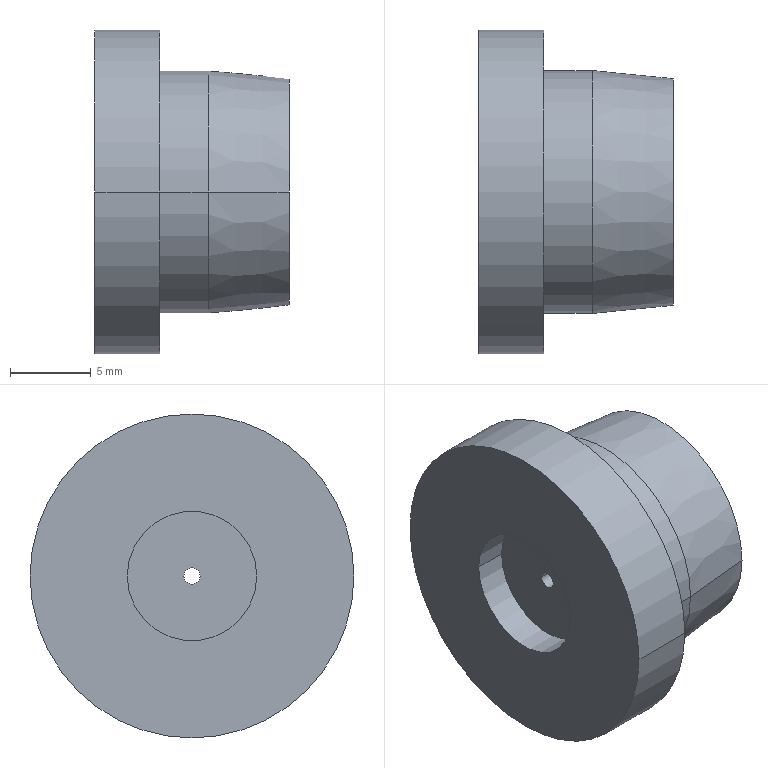Part | SolidWorks | features ICE 3, RevCut 1, Revolution 1 | 1 solid | 19 faces | box 12 x 20 x 20 mm | volume 1878 mm3 | cylinder 10 | plane 5 | sphere 2 | cone 2 | commonest cylinder face diameters 1 x2 4 x2 8 x2 15 x2 20 x2
STEP:
#1=CARTESIAN_POINT('',(12.,-5.809,0.));
#2=VERTEX_POINT('',#1);
#3=CARTESIAN_POINT('',(12.,5.809,0.));
#4=VERTEX_POINT('',#3);
#5=CARTESIAN_POINT('',(12.,0.,0.));
#6=DIRECTION('',(-1.,0.,0.));
#7=DIRECTION('',(0.,1.,0.));
#8=AXIS2_PLACEMENT_3D('',#5,#6,#7);
#9=CIRCLE('',#8,5.809);
#10=EDGE_CURVE('',#2,#4,#9,.T.);
#11=ORIENTED_EDGE('',*,*,#10,.F.);
#12=CARTESIAN_POINT('',(4.843,-2.,0.));
#13=VERTEX_POINT('',#12);
#14=CARTESIAN_POINT('',(10.5,0.,0.));
#15=DIRECTION('',(0.,0.,-1.));
#16=DIRECTION('',(0.,1.,0.));
#17=AXIS2_PLACEMENT_3D('',#14,#15,#16);
#18=CIRCLE('',#17,6.);
#19=EDGE_CURVE('',#2,#13,#18,.T.);
#20=ORIENTED_EDGE('',*,*,#19,.T.);
#21=CARTESIAN_POINT('',(4.843,2.,0.));
#22=VERTEX_POINT('',#21);
#23=CARTESIAN_POINT('',(4.843,0.,0.));
#24=DIRECTION('',(-1.,0.,0.));
#25=DIRECTION('',(0.,1.,0.));
#26=AXIS2_PLACEMENT_3D('',#23,#24,#25);
#27=CIRCLE('',#26,2.);
#28=EDGE_CURVE('',#13,#22,#27,.T.);
#29=ORIENTED_EDGE('',*,*,#28,.T.);
#30=CARTESIAN_POINT('',(10.5,0.,0.));
#31=DIRECTION('',(0.,0.,1.));
#32=DIRECTION('',(0.,-1.,0.));
#33=AXIS2_PLACEMENT_3D('',#30,#31,#32);
#34=CIRCLE('',#33,6.);
#35=EDGE_CURVE('',#4,#22,#34,.T.);
#36=ORIENTED_EDGE('',*,*,#35,.F.);
#37=EDGE_LOOP('',(#11,#20,#29,#36));
#38=FACE_OUTER_BOUND('',#37,.T.);
#39=CARTESIAN_POINT('',(10.5,0.,0.));
#40=DIRECTION('',(0.,0.,-1.));
#41=DIRECTION('',(0.,1.,0.));
#42=AXIS2_PLACEMENT_3D('',#39,#40,#41);
#43=SPHERICAL_SURFACE('',#42,6.);
#44=ADVANCED_FACE('',(#38),#43,.F.);
#45=CARTESIAN_POINT('',(3.5,-0.5,0.));
#46=VERTEX_POINT('',#45);
#47=CARTESIAN_POINT('',(3.5,0.5,0.));
#48=VERTEX_POINT('',#47);
#49=CARTESIAN_POINT('',(3.5,0.,0.));
#50=DIRECTION('',(1.,0.,0.));
#51=DIRECTION('',(0.,-1.,0.));
#52=AXIS2_PLACEMENT_3D('',#49,#50,#51);
#53=CIRCLE('',#52,0.5);
#54=EDGE_CURVE('',#46,#48,#53,.T.);
#55=ORIENTED_EDGE('',*,*,#54,.T.);
#56=CARTESIAN_POINT('',(2.,0.5,0.));
#57=VERTEX_POINT('',#56);
#58=CARTESIAN_POINT('',(17.,0.5,0.));
#59=DIRECTION('',(-1.,0.,0.));
#60=VECTOR('',#59,1000.);
#61=LINE('',#58,#60);
#62=EDGE_CURVE('',#48,#57,#61,.T.);
#63=ORIENTED_EDGE('',*,*,#62,.T.);
#64=CARTESIAN_POINT('',(2.,-0.5,0.));
#65=VERTEX_POINT('',#64);
#66=CARTESIAN_POINT('',(2.,0.,0.));
#67=DIRECTION('',(-1.,0.,0.));
#68=DIRECTION('',(0.,-1.,0.));
#69=AXIS2_PLACEMENT_3D('',#66,#67,#68);
#70=CIRCLE('',#69,0.5);
#71=EDGE_CURVE('',#57,#65,#70,.T.);
#72=ORIENTED_EDGE('',*,*,#71,.T.);
#73=CARTESIAN_POINT('',(17.,-0.5,0.));
#74=DIRECTION('',(-1.,0.,0.));
#75=VECTOR('',#74,1000.);
#76=LINE('',#73,#75);
#77=EDGE_CURVE('',#46,#65,#76,.T.);
#78=ORIENTED_EDGE('',*,*,#77,.F.);
#79=EDGE_LOOP('',(#55,#63,#72,#78));
#80=FACE_OUTER_BOUND('',#79,.T.);
#81=CARTESIAN_POINT('',(17.,0.,0.));
#82=DIRECTION('',(-1.,0.,0.));
#83=DIRECTION('',(0.,-1.,0.));
#84=AXIS2_PLACEMENT_3D('',#81,#82,#83);
#85=CYLINDRICAL_SURFACE('',#84,0.5);
#86=ADVANCED_FACE('',(#80),#85,.F.);
#87=CARTESIAN_POINT('',(2.,4.,0.));
#88=VERTEX_POINT('',#87);
#89=CARTESIAN_POINT('',(2.,-4.,0.));
#90=VERTEX_POINT('',#89);
#91=CARTESIAN_POINT('',(2.,0.,0.));
#92=DIRECTION('',(-1.,0.,0.));
#93=DIRECTION('',(0.,-1.,0.));
#94=AXIS2_PLACEMENT_3D('',#91,#92,#93);
#95=CIRCLE('',#94,4.);
#96=EDGE_CURVE('',#88,#90,#95,.T.);
#97=ORIENTED_EDGE('',*,*,#96,.F.);
#98=CARTESIAN_POINT('',(0.,4.,0.));
#99=VERTEX_POINT('',#98);
#100=CARTESIAN_POINT('',(2.,4.,0.));
#101=DIRECTION('',(-1.,0.,0.));
#102=VECTOR('',#101,1000.);
#103=LINE('',#100,#102);
#104=EDGE_CURVE('',#88,#99,#103,.T.);
#105=ORIENTED_EDGE('',*,*,#104,.T.);
#106=CARTESIAN_POINT('',(0.,-4.,0.));
#107=VERTEX_POINT('',#106);
#108=CARTESIAN_POINT('',(0.,0.,0.));
#109=DIRECTION('',(-1.,0.,0.));
#110=DIRECTION('',(0.,-1.,0.));
#111=AXIS2_PLACEMENT_3D('',#108,#109,#110);
#112=CIRCLE('',#111,4.);
#113=EDGE_CURVE('',#99,#107,#112,.T.);
#114=ORIENTED_EDGE('',*,*,#113,.T.);
#115=CARTESIAN_POINT('',(2.,-4.,0.));
#116=DIRECTION('',(-1.,0.,0.));
#117=VECTOR('',#116,1000.);
#118=LINE('',#115,#117);
#119=EDGE_CURVE('',#90,#107,#118,.T.);
#120=ORIENTED_EDGE('',*,*,#119,.F.);
#121=EDGE_LOOP('',(#97,#105,#114,#120));
#122=FACE_OUTER_BOUND('',#121,.T.);
#123=CARTESIAN_POINT('',(2.,0.,0.));
#124=DIRECTION('',(-1.,0.,0.));
#125=DIRECTION('',(0.,-1.,0.));
#126=AXIS2_PLACEMENT_3D('',#123,#124,#125);
#127=CYLINDRICAL_SURFACE('',#126,4.);
#128=ADVANCED_FACE('',(#122),#127,.F.);
#129=CARTESIAN_POINT('',(12.,7.,0.));
#130=VERTEX_POINT('',#129);
#131=CARTESIAN_POINT('',(12.,-7.,0.));
#132=VERTEX_POINT('',#131);
#133=CARTESIAN_POINT('',(12.,0.,0.));
#134=DIRECTION('',(1.,0.,0.));
#135=DIRECTION('',(0.,1.,0.));
#136=AXIS2_PLACEMENT_3D('',#133,#134,#135);
#137=CIRCLE('',#136,7.);
#138=EDGE_CURVE('',#130,#132,#137,.T.);
#139=ORIENTED_EDGE('',*,*,#138,.F.);
#140=CARTESIAN_POINT('',(7.,7.5,0.));
#141=VERTEX_POINT('',#140);
#142=CARTESIAN_POINT('',(12.,7.,0.));
#143=DIRECTION('',(-0.995,0.0995,0.));
#144=VECTOR('',#143,1000.);
#145=LINE('',#142,#144);
#146=EDGE_CURVE('',#130,#141,#145,.T.);
#147=ORIENTED_EDGE('',*,*,#146,.T.);
#148=CARTESIAN_POINT('',(7.,-7.5,0.));
#149=VERTEX_POINT('',#148);
#150=CARTESIAN_POINT('',(7.,0.,0.));
#151=DIRECTION('',(1.,0.,0.));
#152=DIRECTION('',(0.,1.,0.));
#153=AXIS2_PLACEMENT_3D('',#150,#151,#152);
#154=CIRCLE('',#153,7.5);
#155=EDGE_CURVE('',#141,#149,#154,.T.);
#156=ORIENTED_EDGE('',*,*,#155,.T.);
#157=CARTESIAN_POINT('',(12.,-7.,0.));
#158=DIRECTION('',(-0.995,-0.0995,0.));
#159=VECTOR('',#158,1000.);
#160=LINE('',#157,#159);
#161=EDGE_CURVE('',#132,#149,#160,.T.);
#162=ORIENTED_EDGE('',*,*,#161,.F.);
#163=EDGE_LOOP('',(#139,#147,#156,#162));
#164=FACE_OUTER_BOUND('',#163,.T.);
#165=CARTESIAN_POINT('',(12.,0.,0.));
#166=DIRECTION('',(-1.,0.,0.));
#167=DIRECTION('',(0.,-1.,0.));
#168=AXIS2_PLACEMENT_3D('',#165,#166,#167);
#169=CONICAL_SURFACE('',#168,7.,0.09967);
#170=ADVANCED_FACE('',(#164),#169,.T.);
#171=CARTESIAN_POINT('',(4.,7.5,0.));
#172=VERTEX_POINT('',#171);
#173=CARTESIAN_POINT('',(4.,-7.5,0.));
#174=VERTEX_POINT('',#173);
#175=CARTESIAN_POINT('',(4.,0.,0.));
#176=DIRECTION('',(1.,0.,0.));
#177=DIRECTION('',(0.,1.,0.));
#178=AXIS2_PLACEMENT_3D('',#175,#176,#177);
#179=CIRCLE('',#178,7.5);
#180=EDGE_CURVE('',#172,#174,#179,.T.);
#181=ORIENTED_EDGE('',*,*,#180,.T.);
#182=CARTESIAN_POINT('',(12.,-7.5,0.));
#183=DIRECTION('',(1.,0.,0.));
#184=VECTOR('',#183,1000.);
#185=LINE('',#182,#184);
#186=EDGE_CURVE('',#174,#149,#185,.T.);
#187=ORIENTED_EDGE('',*,*,#186,.T.);
#188=ORIENTED_EDGE('',*,*,#155,.F.);
#189=CARTESIAN_POINT('',(12.,7.5,0.));
#190=DIRECTION('',(1.,0.,0.));
#191=VECTOR('',#190,1000.);
#192=LINE('',#189,#191);
#193=EDGE_CURVE('',#172,#141,#192,.T.);
#194=ORIENTED_EDGE('',*,*,#193,.F.);
#195=EDGE_LOOP('',(#181,#187,#188,#194));
#196=FACE_OUTER_BOUND('',#195,.T.);
#197=CARTESIAN_POINT('',(12.,0.,0.));
#198=DIRECTION('',(1.,0.,0.));
#199=DIRECTION('',(0.,1.,0.));
#200=AXIS2_PLACEMENT_3D('',#197,#198,#199);
#201=CYLINDRICAL_SURFACE('',#200,7.5);
#202=ADVANCED_FACE('',(#196),#201,.T.);
#203=CARTESIAN_POINT('',(0.,10.,0.));
#204=VERTEX_POINT('',#203);
#205=CARTESIAN_POINT('',(0.,-10.,0.));
#206=VERTEX_POINT('',#205);
#207=CARTESIAN_POINT('',(0.,0.,0.));
#208=DIRECTION('',(1.,0.,0.));
#209=DIRECTION('',(0.,1.,0.));
#210=AXIS2_PLACEMENT_3D('',#207,#208,#209);
#211=CIRCLE('',#210,10.);
#212=EDGE_CURVE('',#204,#206,#211,.T.);
#213=ORIENTED_EDGE('',*,*,#212,.T.);
#214=CARTESIAN_POINT('',(4.,-10.,0.));
#215=VERTEX_POINT('',#214);
#216=CARTESIAN_POINT('',(12.,-10.,0.));
#217=DIRECTION('',(1.,0.,0.));
#218=VECTOR('',#217,1000.);
#219=LINE('',#216,#218);
#220=EDGE_CURVE('',#206,#215,#219,.T.);
#221=ORIENTED_EDGE('',*,*,#220,.T.);
#222=CARTESIAN_POINT('',(4.,10.,0.));
#223=VERTEX_POINT('',#222);
#224=CARTESIAN_POINT('',(4.,0.,0.));
#225=DIRECTION('',(1.,0.,0.));
#226=DIRECTION('',(0.,1.,0.));
#227=AXIS2_PLACEMENT_3D('',#224,#225,#226);
#228=CIRCLE('',#227,10.);
#229=EDGE_CURVE('',#223,#215,#228,.T.);
#230=ORIENTED_EDGE('',*,*,#229,.F.);
#231=CARTESIAN_POINT('',(12.,10.,0.));
#232=DIRECTION('',(1.,0.,0.));
#233=VECTOR('',#232,1000.);
#234=LINE('',#231,#233);
#235=EDGE_CURVE('',#204,#223,#234,.T.);
#236=ORIENTED_EDGE('',*,*,#235,.F.);
#237=EDGE_LOOP('',(#213,#221,#230,#236));
#238=FACE_OUTER_BOUND('',#237,.T.);
#239=CARTESIAN_POINT('',(12.,0.,0.));
#240=DIRECTION('',(1.,0.,0.));
#241=DIRECTION('',(0.,1.,0.));
#242=AXIS2_PLACEMENT_3D('',#239,#240,#241);
#243=CYLINDRICAL_SURFACE('',#242,10.);
#244=ADVANCED_FACE('',(#238),#243,.T.);
#245=CARTESIAN_POINT('',(4.843,0.,0.));
#246=DIRECTION('',(-1.,0.,0.));
#247=DIRECTION('',(0.,1.,0.));
#248=AXIS2_PLACEMENT_3D('',#245,#246,#247);
#249=CIRCLE('',#248,2.);
#250=EDGE_CURVE('',#22,#13,#249,.T.);
#251=ORIENTED_EDGE('',*,*,#250,.F.);
#252=CARTESIAN_POINT('',(3.5,2.,0.));
#253=VERTEX_POINT('',#252);
#254=CARTESIAN_POINT('',(18.5,2.,0.));
#255=DIRECTION('',(-1.,0.,0.));
#256=VECTOR('',#255,1000.);
#257=LINE('',#254,#256);
#258=EDGE_CURVE('',#22,#253,#257,.T.);
#259=ORIENTED_EDGE('',*,*,#258,.T.);
#260=CARTESIAN_POINT('',(3.5,-2.,0.));
#261=VERTEX_POINT('',#260);
#262=CARTESIAN_POINT('',(3.5,0.,0.));
#263=DIRECTION('',(-1.,0.,0.));
#264=DIRECTION('',(0.,-1.,0.));
#265=AXIS2_PLACEMENT_3D('',#262,#263,#264);
#266=CIRCLE('',#265,2.);
#267=EDGE_CURVE('',#253,#261,#266,.T.);
#268=ORIENTED_EDGE('',*,*,#267,.T.);
#269=CARTESIAN_POINT('',(18.5,-2.,0.));
#270=DIRECTION('',(-1.,0.,0.));
#271=VECTOR('',#270,1000.);
#272=LINE('',#269,#271);
#273=EDGE_CURVE('',#13,#261,#272,.T.);
#274=ORIENTED_EDGE('',*,*,#273,.F.);
#275=EDGE_LOOP('',(#251,#259,#268,#274));
#276=FACE_OUTER_BOUND('',#275,.T.);
#277=CARTESIAN_POINT('',(18.5,0.,0.));
#278=DIRECTION('',(-1.,0.,0.));
#279=DIRECTION('',(0.,-1.,0.));
#280=AXIS2_PLACEMENT_3D('',#277,#278,#279);
#281=CYLINDRICAL_SURFACE('',#280,2.);
#282=ADVANCED_FACE('',(#276),#281,.F.);
#283=ORIENTED_EDGE('',*,*,#258,.F.);
#284=ORIENTED_EDGE('',*,*,#28,.F.);
#285=ORIENTED_EDGE('',*,*,#273,.T.);
#286=CARTESIAN_POINT('',(3.5,0.,0.));
#287=DIRECTION('',(-1.,0.,0.));
#288=DIRECTION('',(0.,-1.,0.));
#289=AXIS2_PLACEMENT_3D('',#286,#287,#288);
#290=CIRCLE('',#289,2.);
#291=EDGE_CURVE('',#261,#253,#290,.T.);
#292=ORIENTED_EDGE('',*,*,#291,.T.);
#293=EDGE_LOOP('',(#283,#284,#285,#292));
#294=FACE_OUTER_BOUND('',#293,.T.);
#295=CARTESIAN_POINT('',(18.5,0.,0.));
#296=DIRECTION('',(-1.,0.,0.));
#297=DIRECTION('',(0.,-1.,0.));
#298=AXIS2_PLACEMENT_3D('',#295,#296,#297);
#299=CYLINDRICAL_SURFACE('',#298,2.);
#300=ADVANCED_FACE('',(#294),#299,.F.);
#301=CARTESIAN_POINT('',(0.,0.,0.));
#302=DIRECTION('',(-1.,0.,0.));
#303=DIRECTION('',(0.,-1.,0.));
#304=AXIS2_PLACEMENT_3D('',#301,#302,#303);
#305=CIRCLE('',#304,4.);
#306=EDGE_CURVE('',#107,#99,#305,.T.);
#307=ORIENTED_EDGE('',*,*,#306,.F.);
#308=ORIENTED_EDGE('',*,*,#113,.F.);
#309=EDGE_LOOP('',(#307,#308));
#310=FACE_BOUND('',#309,.T.);
#311=ORIENTED_EDGE('',*,*,#212,.F.);
#312=CARTESIAN_POINT('',(0.,0.,0.));
#313=DIRECTION('',(1.,0.,0.));
#314=DIRECTION('',(0.,1.,0.));
#315=AXIS2_PLACEMENT_3D('',#312,#313,#314);
#316=CIRCLE('',#315,10.);
#317=EDGE_CURVE('',#206,#204,#316,.T.);
#318=ORIENTED_EDGE('',*,*,#317,.F.);
#319=EDGE_LOOP('',(#311,#318));
#320=FACE_OUTER_BOUND('',#319,.T.);
#321=CARTESIAN_POINT('',(0.,0.,0.));
#322=DIRECTION('',(-1.,0.,0.));
#323=DIRECTION('',(0.,-1.,0.));
#324=AXIS2_PLACEMENT_3D('',#321,#322,#323);
#325=PLANE('',#324);
#326=ADVANCED_FACE('',(#310,#320),#325,.T.);
#327=ORIENTED_EDGE('',*,*,#220,.F.);
#328=ORIENTED_EDGE('',*,*,#317,.T.);
#329=ORIENTED_EDGE('',*,*,#235,.T.);
#330=CARTESIAN_POINT('',(4.,0.,0.));
#331=DIRECTION('',(1.,0.,0.));
#332=DIRECTION('',(0.,1.,0.));
#333=AXIS2_PLACEMENT_3D('',#330,#331,#332);
#334=CIRCLE('',#333,10.);
#335=EDGE_CURVE('',#215,#223,#334,.T.);
#336=ORIENTED_EDGE('',*,*,#335,.F.);
#337=EDGE_LOOP('',(#327,#328,#329,#336));
#338=FACE_OUTER_BOUND('',#337,.T.);
#339=CARTESIAN_POINT('',(12.,0.,0.));
#340=DIRECTION('',(1.,0.,0.));
#341=DIRECTION('',(0.,1.,0.));
#342=AXIS2_PLACEMENT_3D('',#339,#340,#341);
#343=CYLINDRICAL_SURFACE('',#342,10.);
#344=ADVANCED_FACE('',(#338),#343,.T.);
#345=ORIENTED_EDGE('',*,*,#229,.T.);
#346=ORIENTED_EDGE('',*,*,#335,.T.);
#347=EDGE_LOOP('',(#345,#346));
#348=FACE_OUTER_BOUND('',#347,.T.);
#349=ORIENTED_EDGE('',*,*,#180,.F.);
#350=CARTESIAN_POINT('',(4.,0.,0.));
#351=DIRECTION('',(1.,0.,0.));
#352=DIRECTION('',(0.,1.,0.));
#353=AXIS2_PLACEMENT_3D('',#350,#351,#352);
#354=CIRCLE('',#353,7.5);
#355=EDGE_CURVE('',#174,#172,#354,.T.);
#356=ORIENTED_EDGE('',*,*,#355,.F.);
#357=EDGE_LOOP('',(#349,#356));
#358=FACE_BOUND('',#357,.T.);
#359=CARTESIAN_POINT('',(4.,10.,0.));
#360=DIRECTION('',(1.,0.,0.));
#361=DIRECTION('',(0.,1.,0.));
#362=AXIS2_PLACEMENT_3D('',#359,#360,#361);
#363=PLANE('',#362);
#364=ADVANCED_FACE('',(#348,#358),#363,.T.);
#365=ORIENTED_EDGE('',*,*,#186,.F.);
#366=ORIENTED_EDGE('',*,*,#355,.T.);
#367=ORIENTED_EDGE('',*,*,#193,.T.);
#368=CARTESIAN_POINT('',(7.,0.,0.));
#369=DIRECTION('',(1.,0.,0.));
#370=DIRECTION('',(0.,1.,0.));
#371=AXIS2_PLACEMENT_3D('',#368,#369,#370);
#372=CIRCLE('',#371,7.5);
#373=EDGE_CURVE('',#149,#141,#372,.T.);
#374=ORIENTED_EDGE('',*,*,#373,.F.);
#375=EDGE_LOOP('',(#365,#366,#367,#374));
#376=FACE_OUTER_BOUND('',#375,.T.);
#377=CARTESIAN_POINT('',(12.,0.,0.));
#378=DIRECTION('',(1.,0.,0.));
#379=DIRECTION('',(0.,1.,0.));
#380=AXIS2_PLACEMENT_3D('',#377,#378,#379);
#381=CYLINDRICAL_SURFACE('',#380,7.5);
#382=ADVANCED_FACE('',(#376),#381,.T.);
#383=ORIENTED_EDGE('',*,*,#146,.F.);
#384=CARTESIAN_POINT('',(12.,0.,0.));
#385=DIRECTION('',(1.,0.,0.));
#386=DIRECTION('',(0.,1.,0.));
#387=AXIS2_PLACEMENT_3D('',#384,#385,#386);
#388=CIRCLE('',#387,7.);
#389=EDGE_CURVE('',#132,#130,#388,.T.);
#390=ORIENTED_EDGE('',*,*,#389,.F.);
#391=ORIENTED_EDGE('',*,*,#161,.T.);
#392=ORIENTED_EDGE('',*,*,#373,.T.);
#393=EDGE_LOOP('',(#383,#390,#391,#392));
#394=FACE_OUTER_BOUND('',#393,.T.);
#395=CARTESIAN_POINT('',(12.,0.,0.));
#396=DIRECTION('',(-1.,0.,0.));
#397=DIRECTION('',(0.,-1.,0.));
#398=AXIS2_PLACEMENT_3D('',#395,#396,#397);
#399=CONICAL_SURFACE('',#398,7.,0.09967);
#400=ADVANCED_FACE('',(#394),#399,.T.);
#401=CARTESIAN_POINT('',(12.,0.,0.));
#402=DIRECTION('',(-1.,0.,0.));
#403=DIRECTION('',(0.,1.,0.));
#404=AXIS2_PLACEMENT_3D('',#401,#402,#403);
#405=CIRCLE('',#404,5.809);
#406=EDGE_CURVE('',#4,#2,#405,.T.);
#407=ORIENTED_EDGE('',*,*,#406,.T.);
#408=ORIENTED_EDGE('',*,*,#10,.T.);
#409=EDGE_LOOP('',(#407,#408));
#410=FACE_BOUND('',#409,.T.);
#411=ORIENTED_EDGE('',*,*,#389,.T.);
#412=ORIENTED_EDGE('',*,*,#138,.T.);
#413=EDGE_LOOP('',(#411,#412));
#414=FACE_OUTER_BOUND('',#413,.T.);
#415=CARTESIAN_POINT('',(12.,7.,0.));
#416=DIRECTION('',(1.,0.,0.));
#417=DIRECTION('',(0.,1.,0.));
#418=AXIS2_PLACEMENT_3D('',#415,#416,#417);
#419=PLANE('',#418);
#420=ADVANCED_FACE('',(#410,#414),#419,.T.);
#421=ORIENTED_EDGE('',*,*,#104,.F.);
#422=CARTESIAN_POINT('',(2.,0.,0.));
#423=DIRECTION('',(-1.,0.,0.));
#424=DIRECTION('',(0.,-1.,0.));
#425=AXIS2_PLACEMENT_3D('',#422,#423,#424);
#426=CIRCLE('',#425,4.);
#427=EDGE_CURVE('',#90,#88,#426,.T.);
#428=ORIENTED_EDGE('',*,*,#427,.F.);
#429=ORIENTED_EDGE('',*,*,#119,.T.);
#430=ORIENTED_EDGE('',*,*,#306,.T.);
#431=EDGE_LOOP('',(#421,#428,#429,#430));
#432=FACE_OUTER_BOUND('',#431,.T.);
#433=CARTESIAN_POINT('',(2.,0.,0.));
#434=DIRECTION('',(-1.,0.,0.));
#435=DIRECTION('',(0.,-1.,0.));
#436=AXIS2_PLACEMENT_3D('',#433,#434,#435);
#437=CYLINDRICAL_SURFACE('',#436,4.);
#438=ADVANCED_FACE('',(#432),#437,.F.);
#439=CARTESIAN_POINT('',(2.,0.,0.));
#440=DIRECTION('',(-1.,0.,0.));
#441=DIRECTION('',(0.,-1.,0.));
#442=AXIS2_PLACEMENT_3D('',#439,#440,#441);
#443=CIRCLE('',#442,0.5);
#444=EDGE_CURVE('',#65,#57,#443,.T.);
#445=ORIENTED_EDGE('',*,*,#444,.F.);
#446=ORIENTED_EDGE('',*,*,#71,.F.);
#447=EDGE_LOOP('',(#445,#446));
#448=FACE_BOUND('',#447,.T.);
#449=ORIENTED_EDGE('',*,*,#427,.T.);
#450=ORIENTED_EDGE('',*,*,#96,.T.);
#451=EDGE_LOOP('',(#449,#450));
#452=FACE_OUTER_BOUND('',#451,.T.);
#453=CARTESIAN_POINT('',(2.,0.,0.));
#454=DIRECTION('',(-1.,0.,0.));
#455=DIRECTION('',(0.,-1.,0.));
#456=AXIS2_PLACEMENT_3D('',#453,#454,#455);
#457=PLANE('',#456);
#458=ADVANCED_FACE('',(#448,#452),#457,.T.);
#459=ORIENTED_EDGE('',*,*,#62,.F.);
#460=CARTESIAN_POINT('',(3.5,0.,0.));
#461=DIRECTION('',(1.,0.,0.));
#462=DIRECTION('',(0.,-1.,0.));
#463=AXIS2_PLACEMENT_3D('',#460,#461,#462);
#464=CIRCLE('',#463,0.5);
#465=EDGE_CURVE('',#48,#46,#464,.T.);
#466=ORIENTED_EDGE('',*,*,#465,.T.);
#467=ORIENTED_EDGE('',*,*,#77,.T.);
#468=ORIENTED_EDGE('',*,*,#444,.T.);
#469=EDGE_LOOP('',(#459,#466,#467,#468));
#470=FACE_OUTER_BOUND('',#469,.T.);
#471=CARTESIAN_POINT('',(17.,0.,0.));
#472=DIRECTION('',(-1.,0.,0.));
#473=DIRECTION('',(0.,-1.,0.));
#474=AXIS2_PLACEMENT_3D('',#471,#472,#473);
#475=CYLINDRICAL_SURFACE('',#474,0.5);
#476=ADVANCED_FACE('',(#470),#475,.F.);
#477=ORIENTED_EDGE('',*,*,#291,.F.);
#478=ORIENTED_EDGE('',*,*,#267,.F.);
#479=EDGE_LOOP('',(#477,#478));
#480=FACE_OUTER_BOUND('',#479,.T.);
#481=ORIENTED_EDGE('',*,*,#54,.F.);
#482=ORIENTED_EDGE('',*,*,#465,.F.);
#483=EDGE_LOOP('',(#481,#482));
#484=FACE_BOUND('',#483,.T.);
#485=CARTESIAN_POINT('',(3.5,0.,0.));
#486=DIRECTION('',(-1.,0.,0.));
#487=DIRECTION('',(0.,-1.,0.));
#488=AXIS2_PLACEMENT_3D('',#485,#486,#487);
#489=PLANE('',#488);
#490=ADVANCED_FACE('',(#480,#484),#489,.F.);
#491=ORIENTED_EDGE('',*,*,#19,.F.);
#492=ORIENTED_EDGE('',*,*,#406,.F.);
#493=ORIENTED_EDGE('',*,*,#35,.T.);
#494=ORIENTED_EDGE('',*,*,#250,.T.);
#495=EDGE_LOOP('',(#491,#492,#493,#494));
#496=FACE_OUTER_BOUND('',#495,.T.);
#497=CARTESIAN_POINT('',(10.5,0.,0.));
#498=DIRECTION('',(0.,0.,-1.));
#499=DIRECTION('',(0.,1.,0.));
#500=AXIS2_PLACEMENT_3D('',#497,#498,#499);
#501=SPHERICAL_SURFACE('',#500,6.);
#502=ADVANCED_FACE('',(#496),#501,.F.);
#503=CLOSED_SHELL('',(#44,#86,#128,#170,#202,#244,#282,#300,#326,#344,#364,#382,#400,#420,#438,#458,#476,#490,#502));
#504=MANIFOLD_SOLID_BREP('',#503);
#505=CARTESIAN_POINT('',(0.,0.,0.));
#506=DIRECTION('',(0.,0.,1.));
#507=DIRECTION('',(1.,0.,0.));
#508=AXIS2_PLACEMENT_3D('',#505,#506,#507);
#509=(LENGTH_UNIT()NAMED_UNIT(*)SI_UNIT(.MILLI.,.METRE.));
#510=UNCERTAINTY_MEASURE_WITH_UNIT(LENGTH_MEASURE(0.00001),#509,'','');
#511=(NAMED_UNIT(*)PLANE_ANGLE_UNIT()SI_UNIT($,.RADIAN.));
#512=(NAMED_UNIT(*)SI_UNIT($,.STERADIAN.)SOLID_ANGLE_UNIT());
#513=(GEOMETRIC_REPRESENTATION_CONTEXT(3)GLOBAL_UNCERTAINTY_ASSIGNED_CONTEXT((#510))GLOBAL_UNIT_ASSIGNED_CONTEXT((#509,#511,#512))REPRESENTATION_CONTEXT('',''));
#514=ADVANCED_BREP_SHAPE_REPRESENTATION('',(#504,#508),#513);